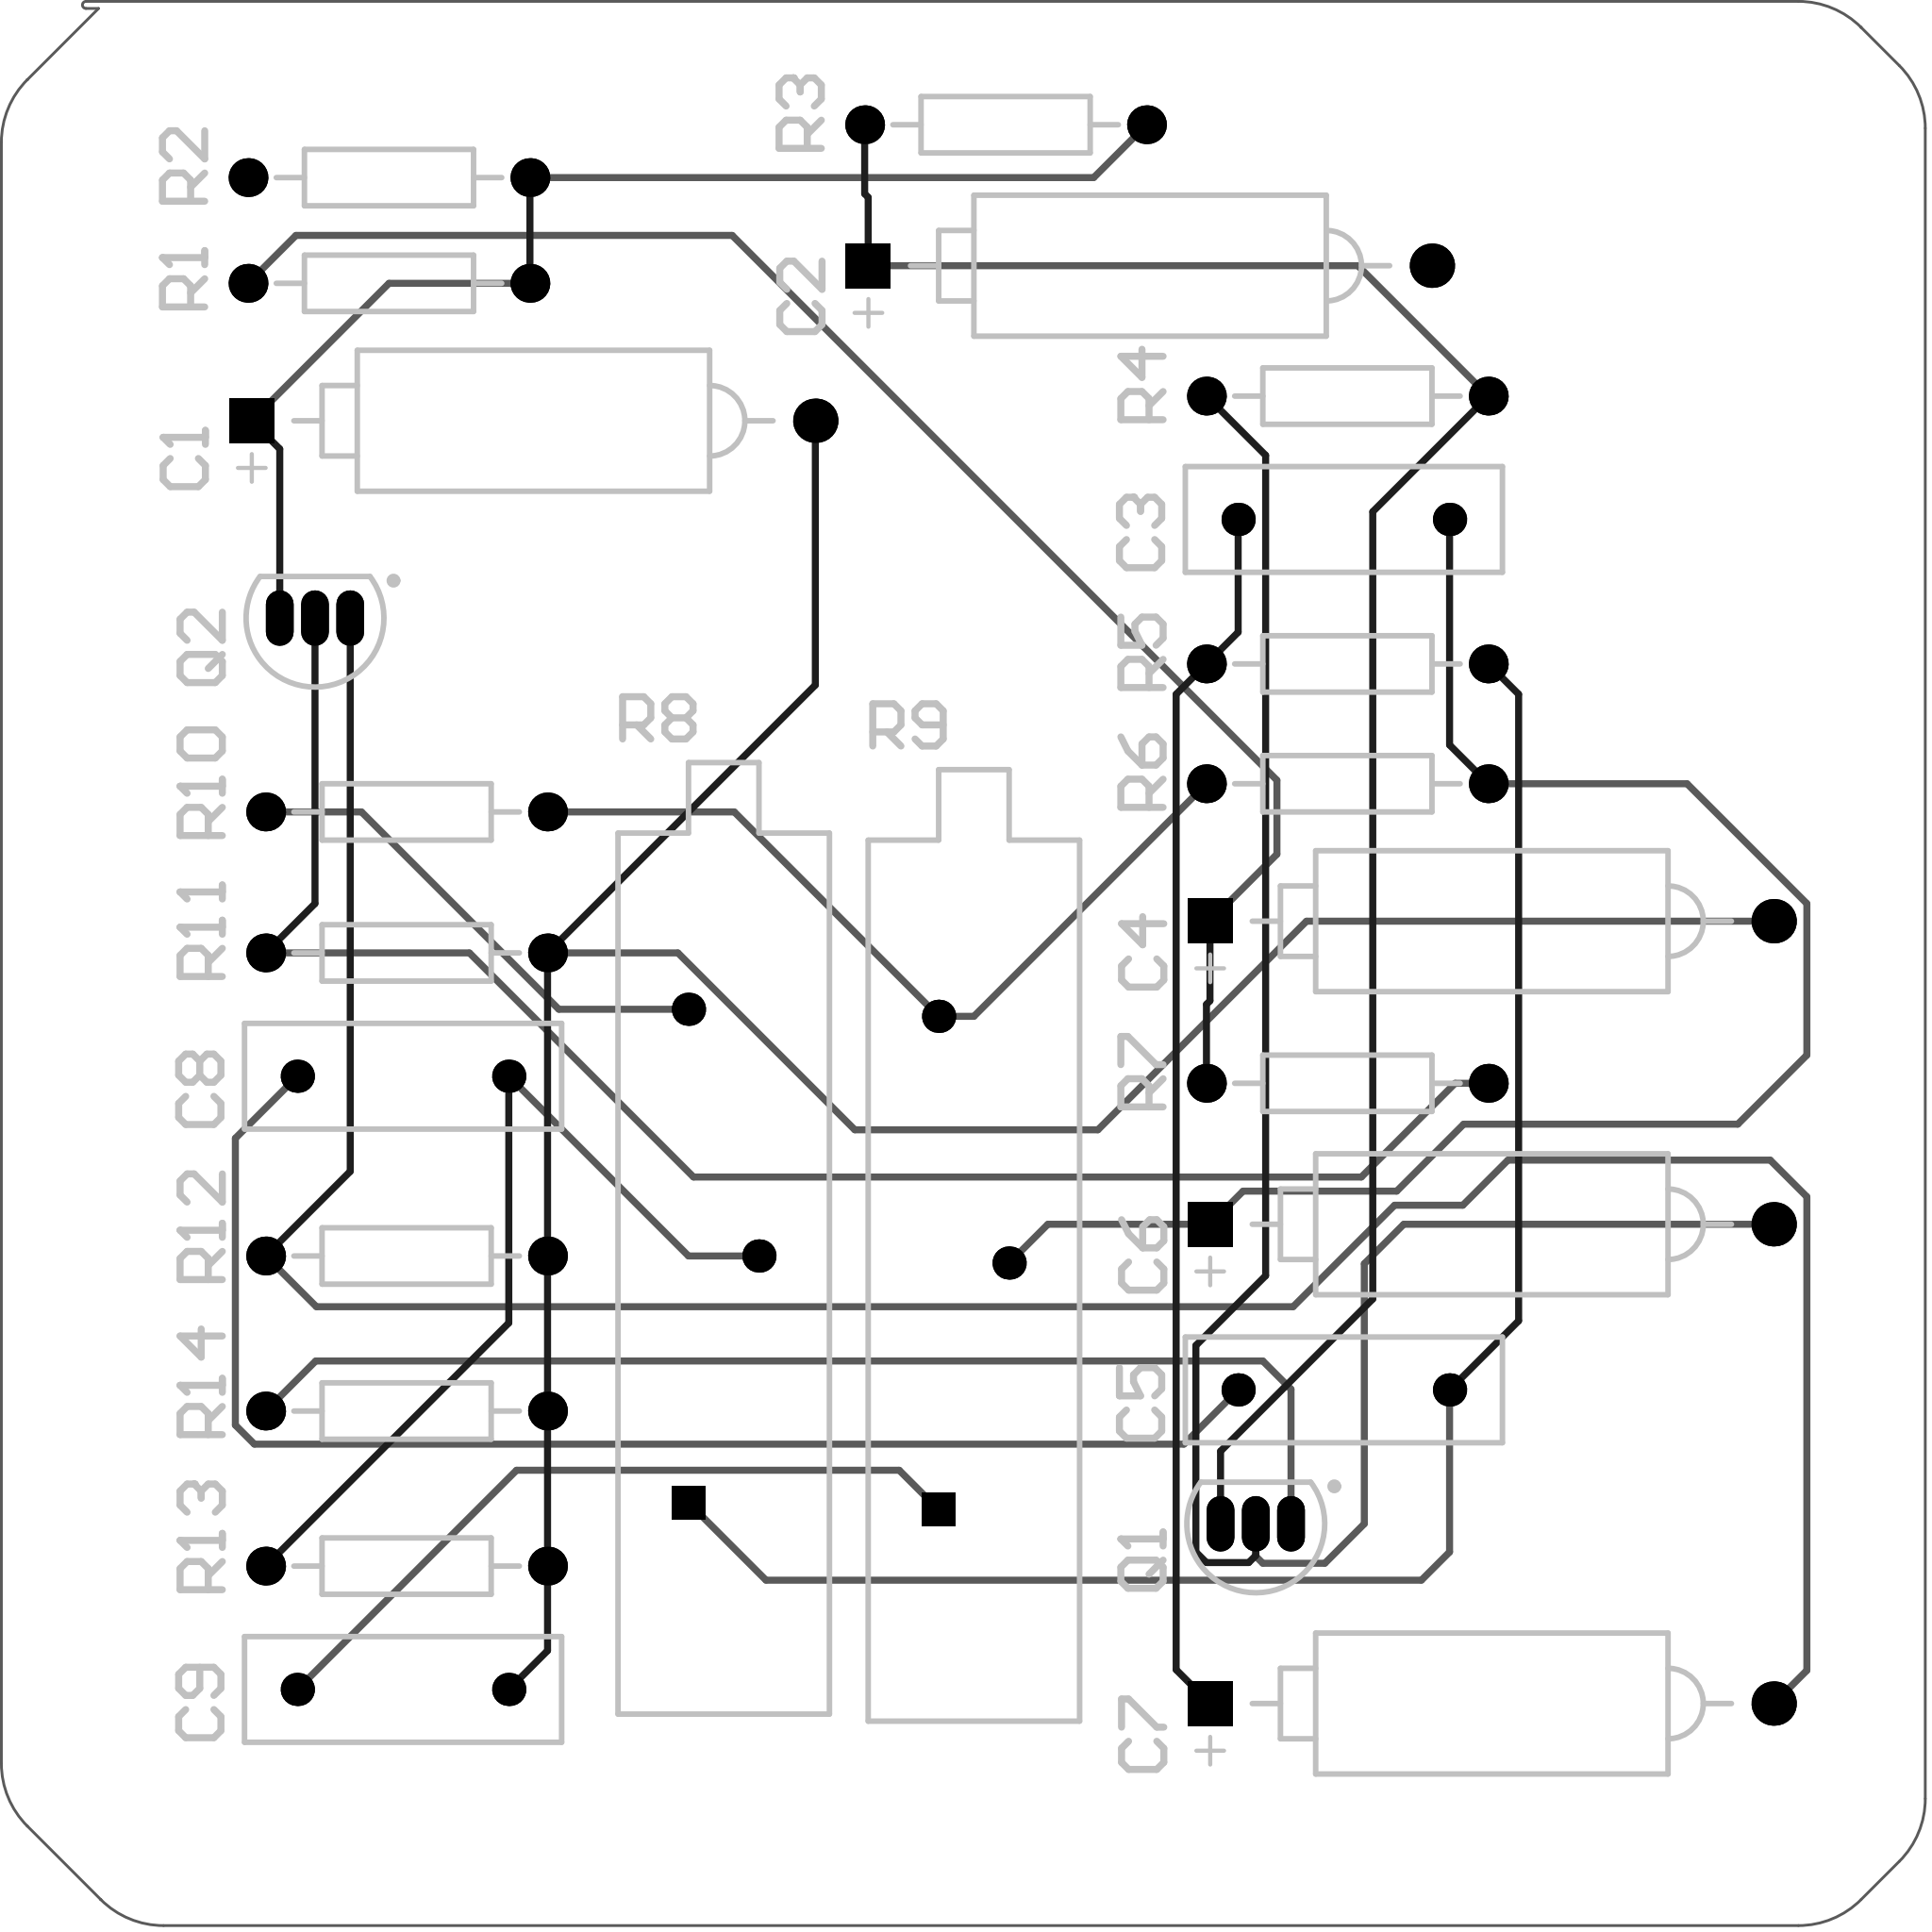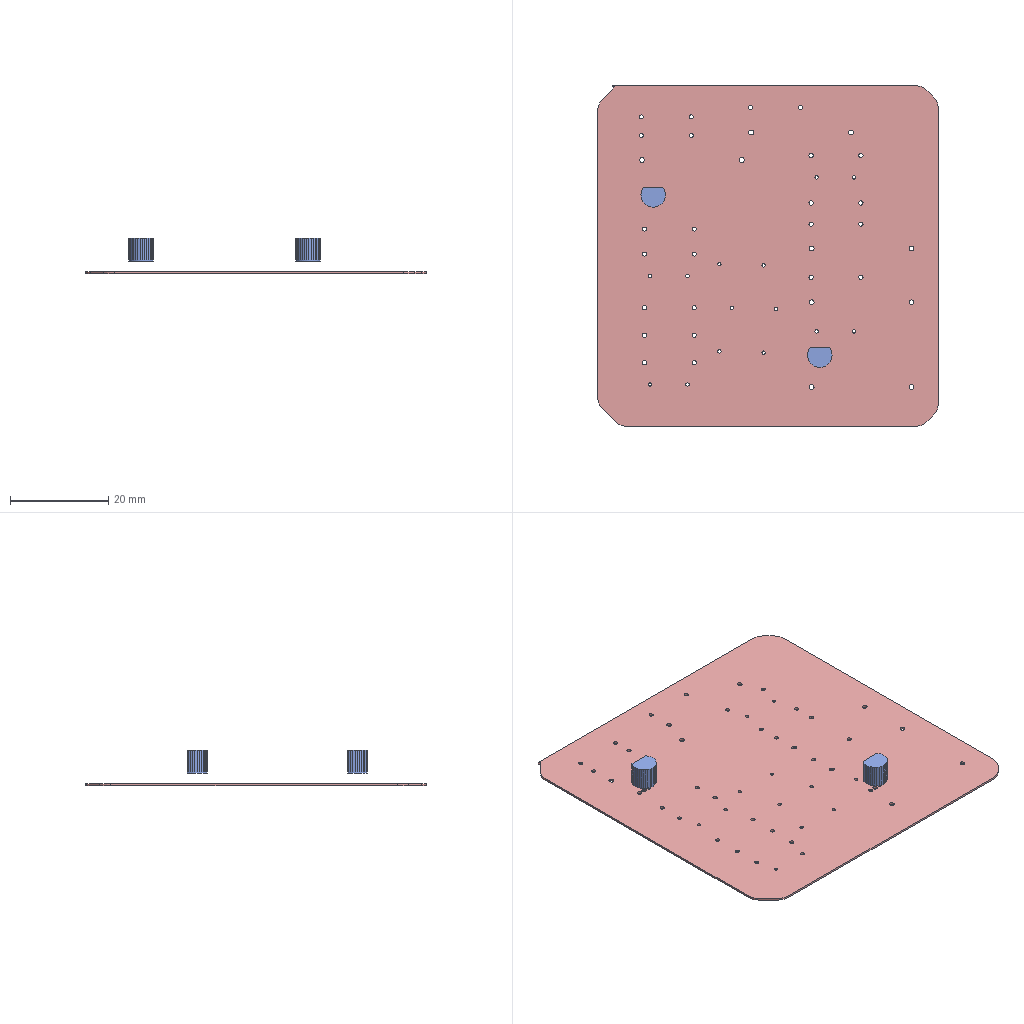Circuit board layout | Altium Designer | box 69.3 x 69.3 x 7.3 mm
Part placement:
Designator,Comment,Layer,Footprint,Center-X(mm),Center-Y(mm),Rotation
R14,Res2,TopLayer,AXIAL-0.4,58.547,69.088,180
R13,Res2,TopLayer,AXIAL-0.4,58.547,63.5,180
R12,Res2,TopLayer,AXIAL-0.4,58.547,74.676,180
R11,Res2,TopLayer,AXIAL-0.4,58.547,85.598,180
R10,Res2,TopLayer,AXIAL-0.4,58.547,90.678,180
R9,Res Tap,TopLayer,VR3,78.994,74.422,90
R8,Res Tap,TopLayer,VR3,69.977,74.676,90
R7,Res2,TopLayer,AXIAL-0.4,92.456,80.899,180
R6,Res2,TopLayer,AXIAL-0.4,92.456,91.694,180
R5,Res2,TopLayer,AXIAL-0.4,92.456,96.012,180
R4,Res2,TopLayer,AXIAL-0.4,92.456,105.664,180
R3,Res2,TopLayer,AXIAL-0.4,80.137,115.443,180
R2,Res2,TopLayer,AXIAL-0.4,57.912,113.538,180
R1,Res2,TopLayer,AXIAL-0.4,57.912,109.728,180
Q2,2N3904,TopLayer,TO-92A,55.245,97.663,90
Q1,2N3904,TopLayer,TO-92A,89.154,65.024,90
C9,Cap,TopLayer,RAD-0.3,58.42,59.055,180
C8,Cap,TopLayer,RAD-0.3,58.42,81.153,180
C7,Cap Pol2,TopLayer,POLAR0.8,97.663,58.547,180
C6,Cap Pol2,TopLayer,POLAR0.8,97.663,75.819,180
C5,Cap,TopLayer,RAD-0.3,92.329,69.85,180
C4,Cap Pol2,TopLayer,POLAR0.8,97.663,86.741,180
C3,Cap,TopLayer,RAD-0.3,92.329,101.219,180
C2,Cap Pol2,TopLayer,POLAR0.8,85.344,110.363,180
C1,Cap Pol2,TopLayer,POLAR0.8,63.119,104.775,180